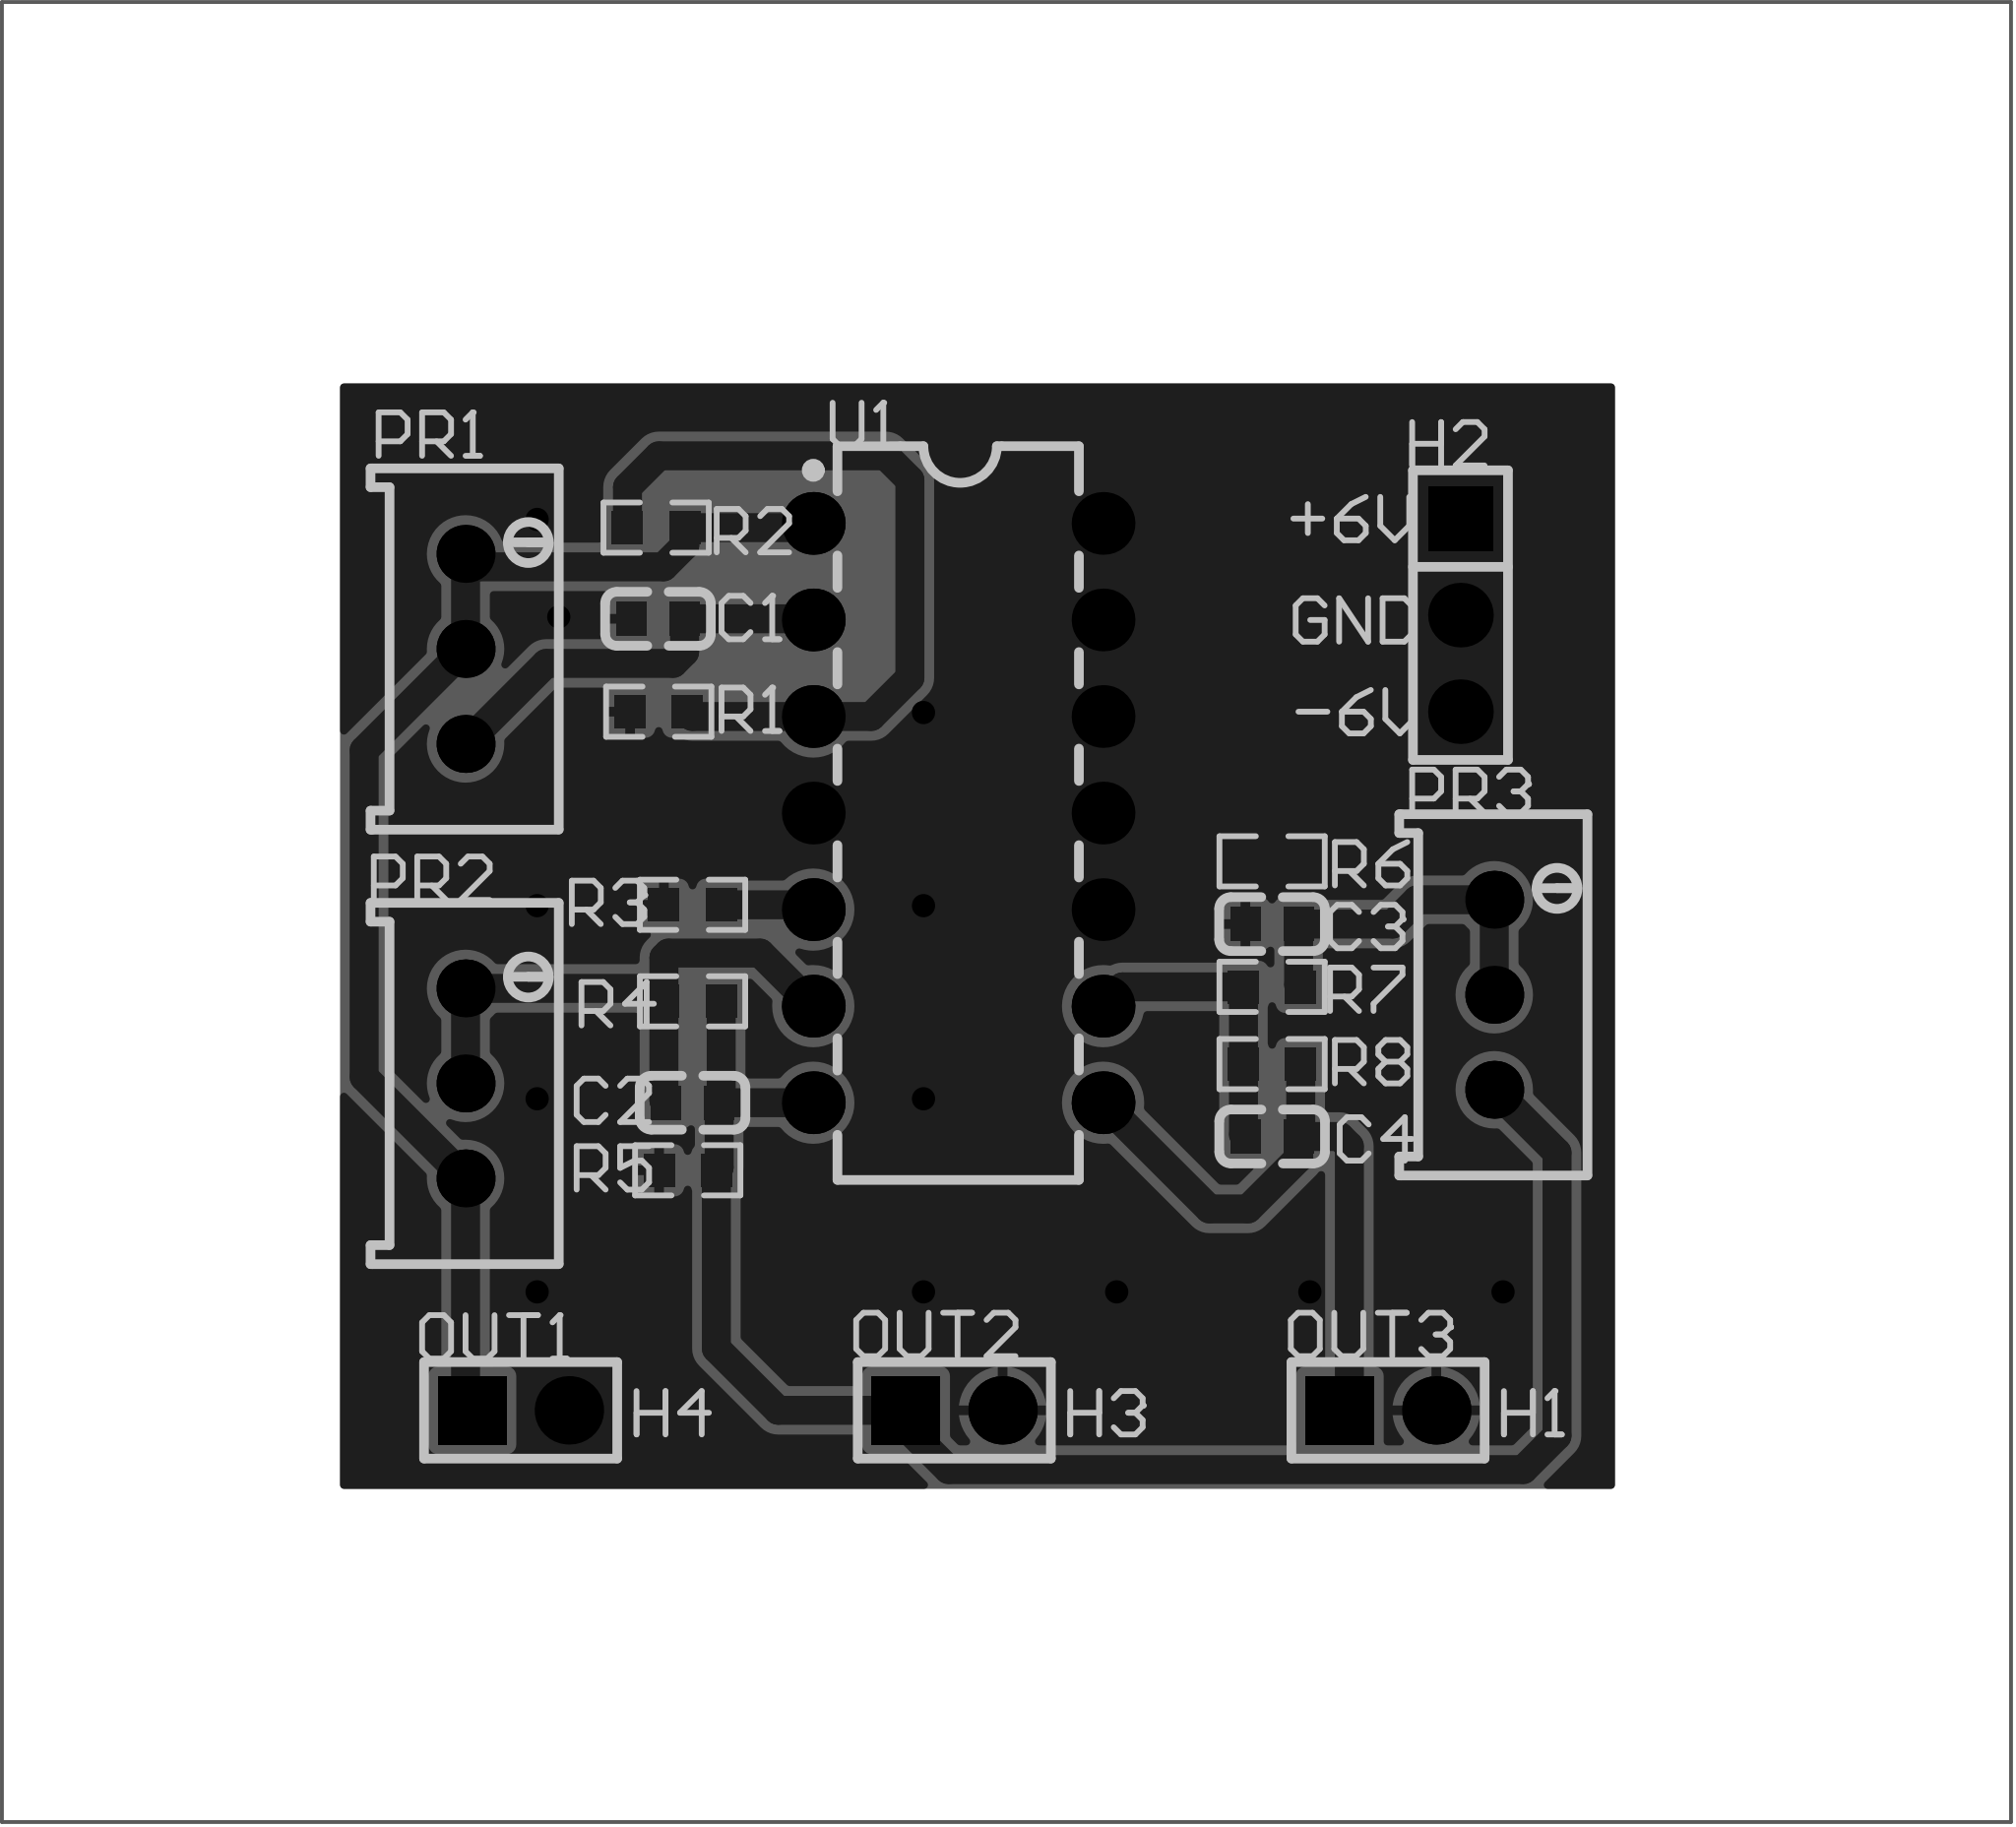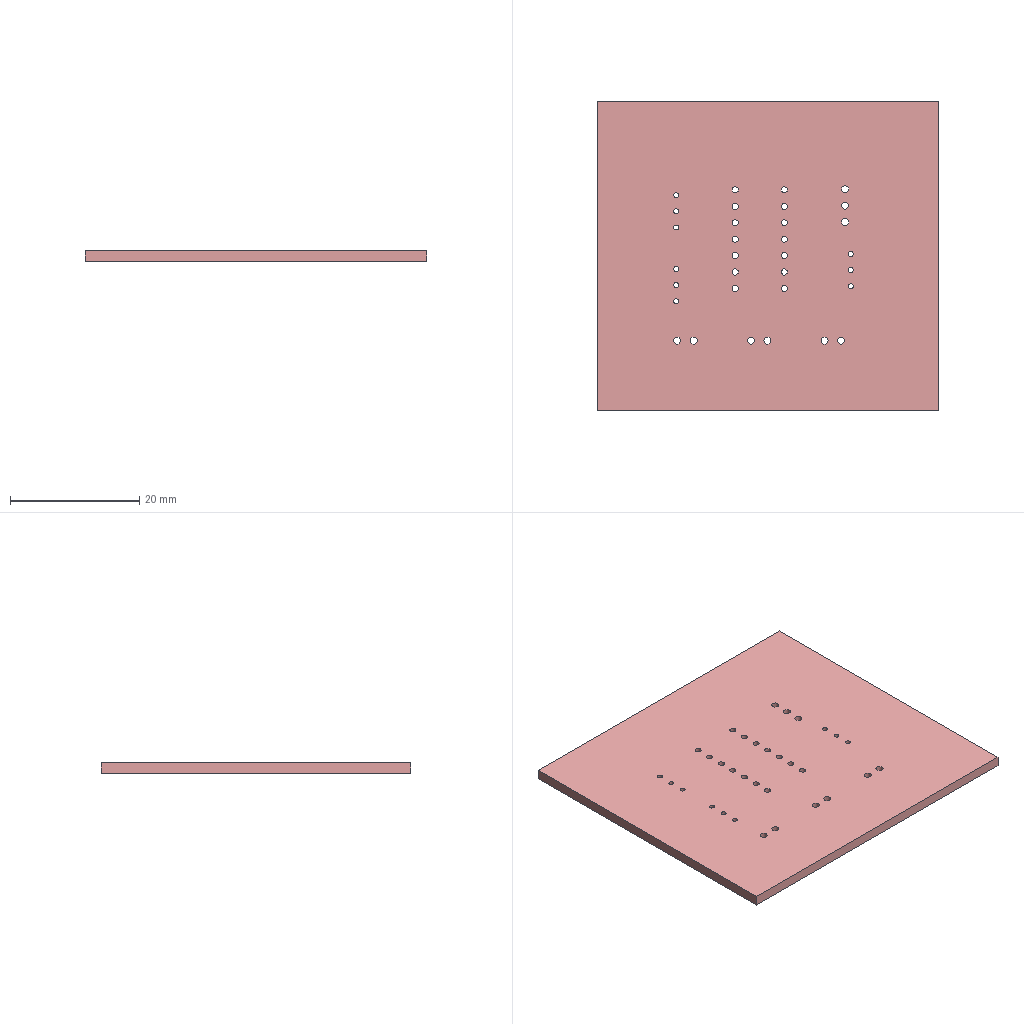Circuit board layout | Altium Designer | box 52.8 x 47.9 x 1.6 mm
Layer stack:
# Altium Designer layer stack of  (unit mm; dielectric type: 0 none, 1 core, 2 prepreg, 3 surface material)
index,name,kind,layer,copper_thickness_mm,dielectric_type,dielectric_thickness_mm,dielectric_material,dielectric_constant
0,Top Paste Mask Layer,other,,,,,,
1,Top Silkscreen Layer,other,,,,,,
2,Top Solder Mask Layer,dielectric,,,3,0.01,,3.3
3,Top Layer,copper,Top Layer,0.035,,,,
4,Dielectric1,dielectric,,,3,1.51,FR4,4.5
5,Bottom Layer,copper,Bottom Layer,0.035,,,,
6,Bottom Solder Mask Layer,dielectric,,,3,0.01,,3.3
7,Bottom Silkscreen Layer,other,,,,,,
8,Bottom Paste Mask Layer,other,,,,,,
# drill layer pairs: low layer,high layer
drill_pair,Top Layer,Bottom Layer
Part placement:
Designator,Comment,Layer,Footprint,Center-X(mm),Center-Y(mm),Rotation
C1,30nF,TopLayer,C0603,87.102,101.504,0
C2,100nF,TopLayer,C0603,88.011,88.773,0
C3,100nF,TopLayer,C0603,103.248,93.472,0
C4,100nF,TopLayer,C0603,103.251,87.884,0
H1,,TopLayer,HDR-TH_2P-P2.54-V-M-1,106.299,80.681,0
H2,,TopLayer,HDR-TH_3P-P2.54-V-M,108.204,101.6,270
PR1,10kΩ,TopLayer,R_3296,82.042,100.711,270
PR2,20kΩ,TopLayer,R_3296,82.042,89.281,270
PR3,200kΩ,TopLayer,R_3296,109.093,91.613,270
R1,10K,TopLayer,R0603,87.122,99.06,0
R2,3.9kΩ,TopLayer,R0603,87.053,103.902,180
R3,100K,TopLayer,R0603,88.011,93.98,0
R4,300K,TopLayer,R0603,88.011,91.44,0
R5,620,TopLayer,R0603,87.884,86.995,0
R6,10K,TopLayer,R0603,103.251,95.123,180
R7,20K,TopLayer,R0603,103.251,91.821,180
R8,24K,TopLayer,R0603,103.251,89.789,0
U1,LM324N/PB,TopLayer,PDIP-14_L19.2-W6.6-P2.54-LS7.6-BL,94.996,96.393,270
H3,,TopLayer,HDR-TH_2P-P2.54-V-M-1,94.894,80.681,0
H4,,TopLayer,HDR-TH_2P-P2.54-V-M-1,83.49,80.681,0
Pad and via stacks:
# Altium Designer via and pad stacks of  (unit mm). Each distinct definition once, with the count of objects using it.
# via: kind,start_layer,end_layer,hole_mm,diameter_mm,mode(0 simple;1 top-mid-bottom;2 full stack),diameter_per_layer,count,example_net
# pad: kind,layer,hole_mm,hole_type(0 round;1 square;2 slot),plating,top_size,top_shape(1 round;2 rect;3 octagon;9 rounded rect),mid_size,bottom_size,mode,footprint,size_per_layer,count,example
pad,Top Layer,0,0,plated,0.8x0.9,2,0.8x0.9,0.8x0.9,0,C0603,,8,C1.2
pad,Top Layer,0,0,plated,0.8065x0.864,2,0.8065x0.864,0.8065x0.864,0,R0603,,16,R1.2
pad,Multi-Layer,1.1,0,plated,1.8x1.8,1,1.8x1.8,1.8x1.8,0,HDR-TH_2P-P2.54-V-M-1,,3,H1.2
pad,Multi-Layer,1.1,0,plated,1.8x1.8,2,1.8x1.8,1.8x1.8,0,HDR-TH_2P-P2.54-V-M-1,,3,H1.1
pad,Multi-Layer,1.1,0,plated,1.7x1.7,2,1.7x1.7,1.7x1.7,0,HDR-TH_3P-P2.54-V-M,,1,H2.1
pad,Multi-Layer,1.1,0,plated,1.7x1.7,1,1.7x1.7,1.7x1.7,0,HDR-TH_3P-P2.54-V-M,,2,H2.2
pad,Multi-Layer,0.762,0,plated,1.524x1.524,1,1.524x1.524,1.524x1.524,0,R_3296,,9,PR1.2
pad,Multi-Layer,0.95,0,plated,1.65x1.65,1,1.65x1.65,1.65x1.65,0,PDIP-14_L19.2-W6.6-P2.54-LS7.6-BL,,14,U1.1
via,Top Layer,Bottom Layer,0.3048,0.61,0,,12,GND
Copper pours:
name,layer,net,type(0 solid;1 hatched;2 none)
Top Layer-GND,Top Layer,GND,0
Bottom Layer-GND,Bottom Layer,GND,0